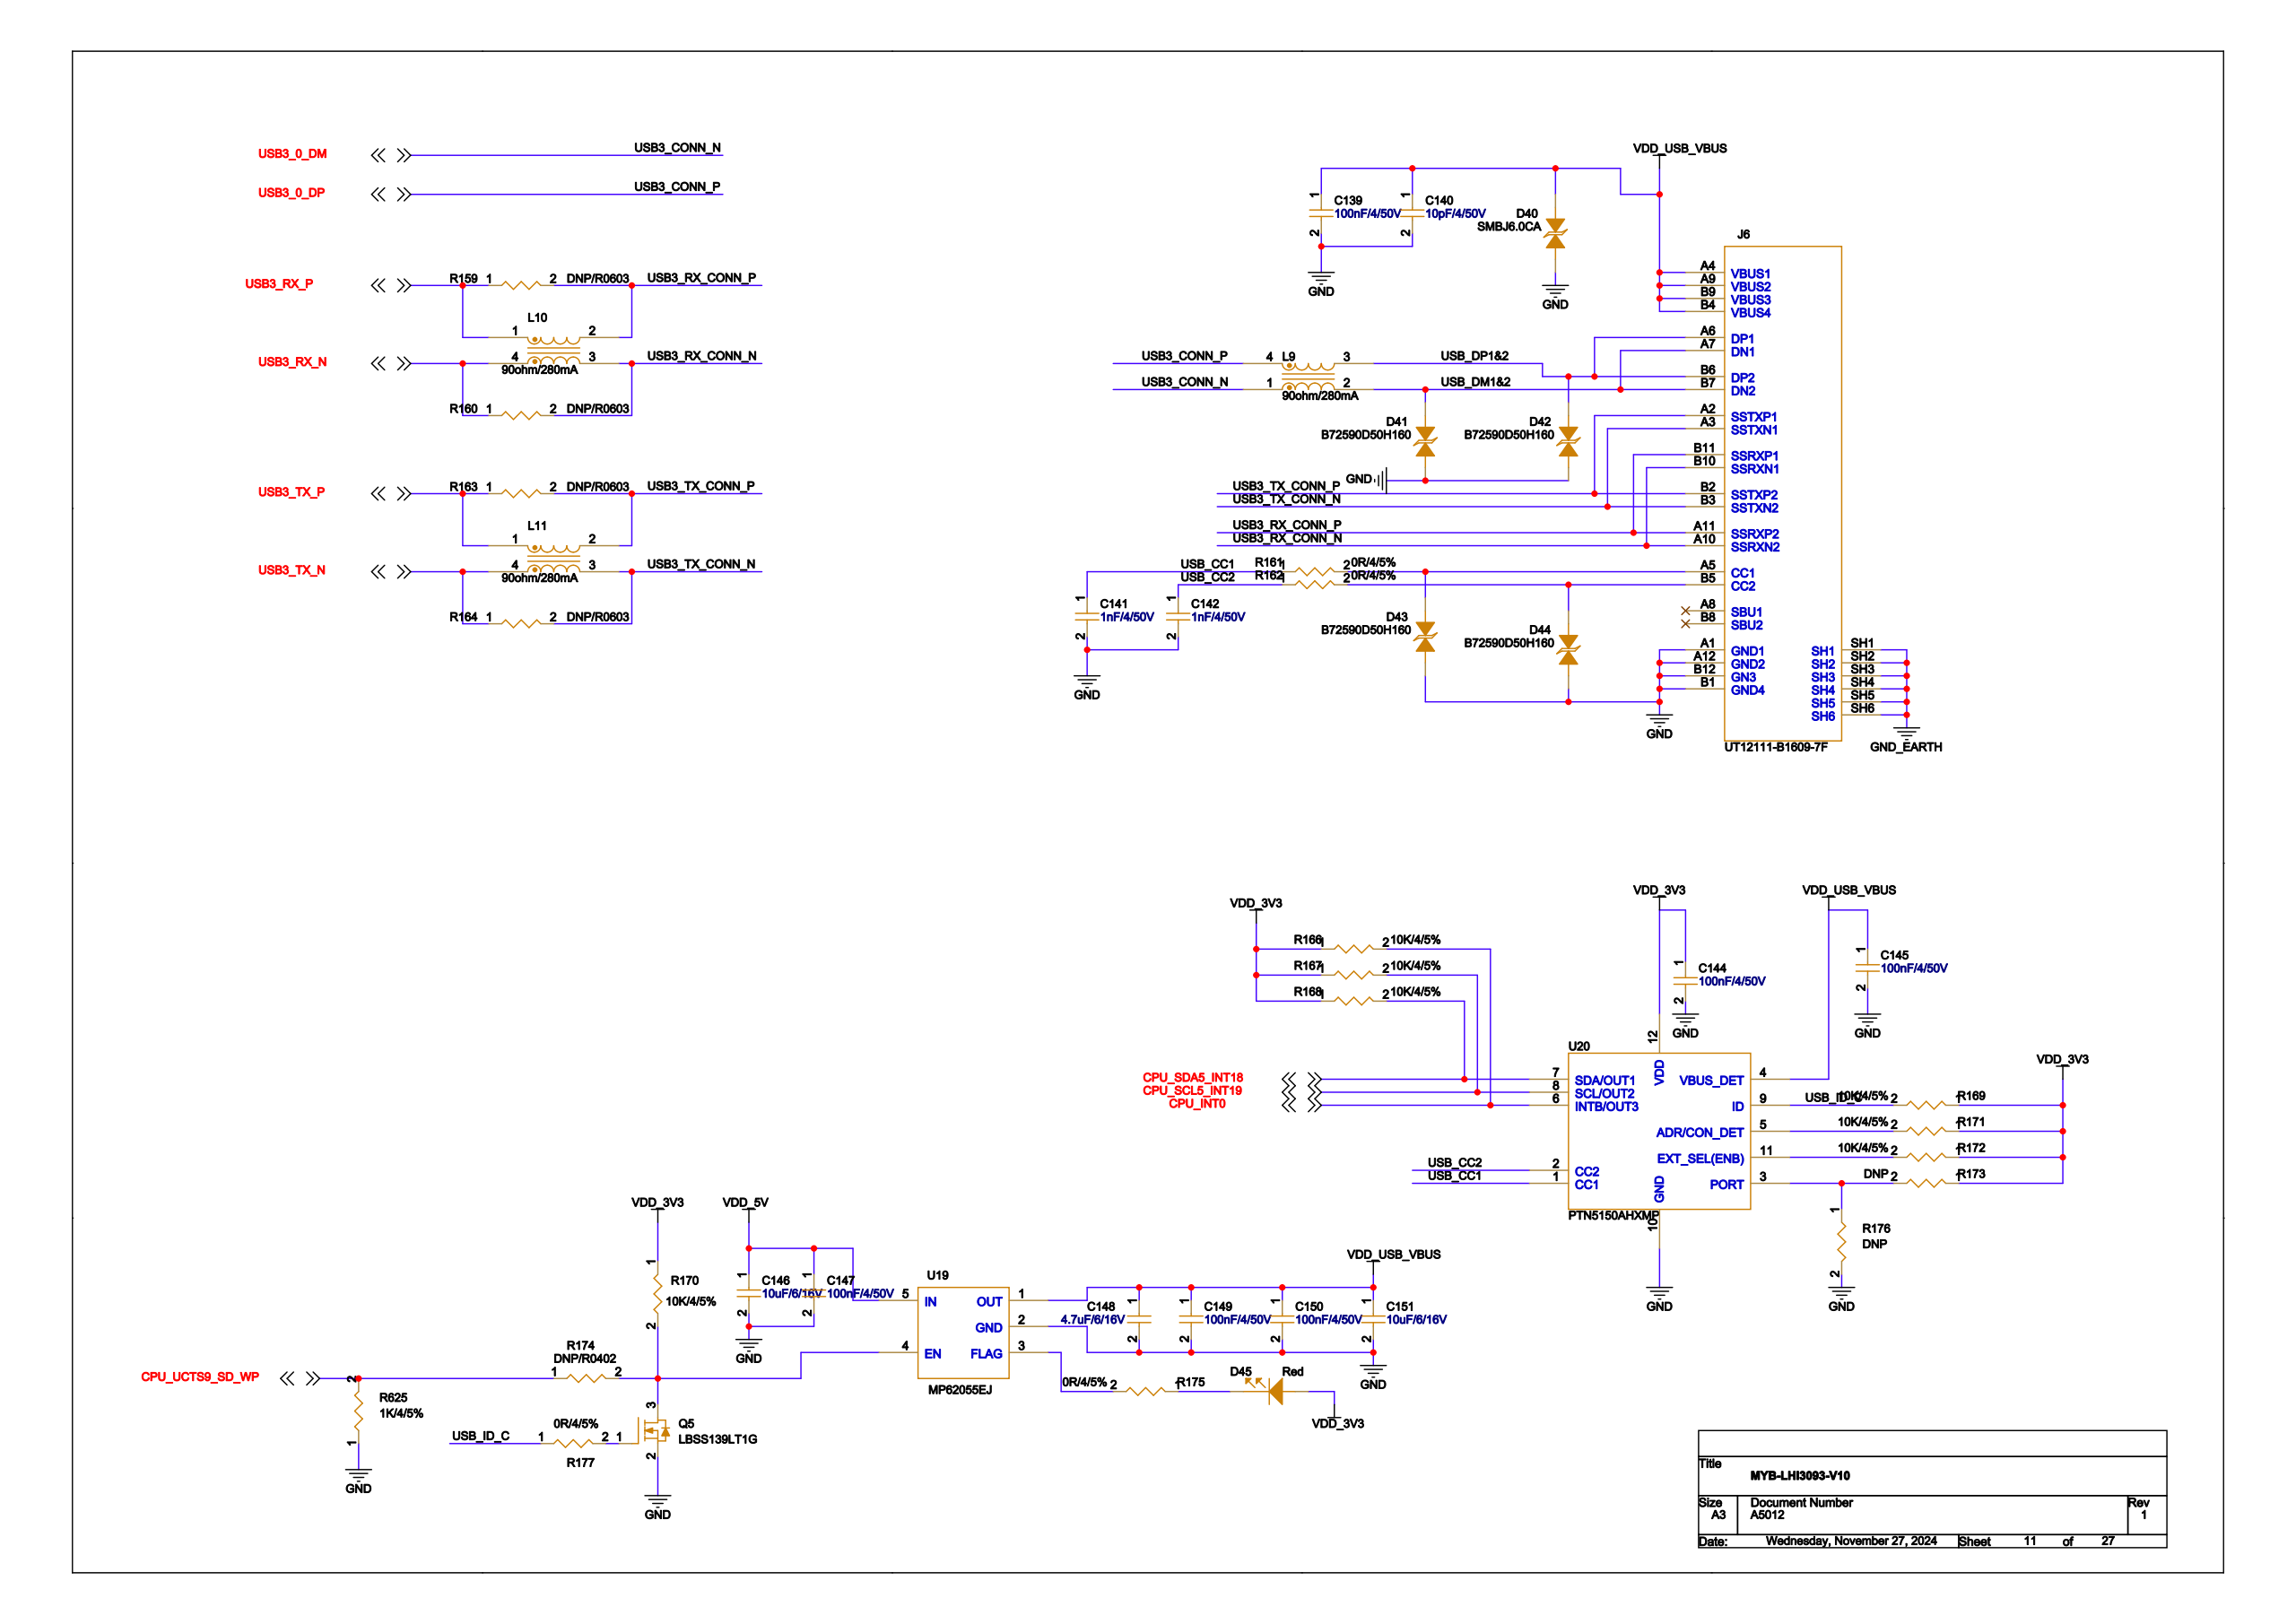Circuit board | Cadence Allegro | 1159 parts | 708 nets | one sheet of the schematic
Parts on this sheet (reference | value | footprint):
C139 | 100nF/4/50V | C0402
C140 | 10pF/4/50V | C0402
C141 | 1nF/4/50V | C0402
C142 | 1nF/4/50V | C0402
C144 | 100nF/4/50V | C0402
C145 | 100nF/4/50V | C0402
C146 | 10uF/6/16V | C0603
C147 | 100nF/4/50V | C0402
C148 | 4.7uF/6/16V | C0603
C149 | 100nF/4/50V | C0402
C150 | 100nF/4/50V | C0402
C151 | 10uF/6/16V | C0603
D40 | SMBJ6.0CA | DO-214AA
D41 | B72590D50H160 | D0402
D42 | B72590D50H160 | D0402
D43 | B72590D50H160 | D0402
D44 | B72590D50H160 | D0402
D45 | LED-SML1206 | LED0603
J6 | UT12111-B1609-7F | UT12111-B1609-7F
L9 | 90ohm/280mA | INDCM-SDCW2012
L10 | 90ohm/280mA | INDCM-SDCW2012
L11 | 90ohm/280mA | INDCM-SDCW2012
Q5 | LBSS139LT1G | SOT-23
R159 | DNP/R0603 | R0603
R160 | DNP/R0603 | R0603
R163 | DNP/R0603 | R0603
R164 | DNP/R0603 | R0603
R170 | 10K/4/5% | R0402
R174 | DNP/R0402 | R0402
R176 | DNP | R0402
R177 | 0R/4/5% | R0402
R625 | 1K/4/5% | R0402
U19 | MP62055EJ | SOT23-5
U20 | PTN5150AHXMP | X2QFN12
Nets of these parts (net: part-pin ...):
GND: C139-2 C140-2 C141-2 C142-2 C144-2 C145-2 C146-2 C147-2 C148-2 C149-2 C150-2 C151-2 D40-1 D41-1 D42-1 D43-1 D44-1 Q5-2 R176-2 R625-1 U19-2 U20-10 J6-A1 J6-A12 J6-B1 J6-B12
VDD_5V: C146-1 C147-1 U19-5
VDD_3V3: C144-1 D45-1 R170-1 U20-12
VDD_USB_VBUS: C139-1 C140-1 C145-1 C148-1 C149-1 C150-1 C151-1 D40-2 U19-1 U20-4 J6-A4 J6-A9 J6-B4 J6-B9
GND_EARTH: J6-SH1 J6-SH2 J6-SH3 J6-SH4 J6-SH5 J6-SH6
USB_CC1: C141-1 U20-1
USB_CC2: C142-1 U20-2
N14881575: D45-2
USB_DM1&2: D41-2 L9-2 J6-A7 J6-B7
USB_DP1&2: D42-2 L9-3 J6-A6 J6-B6
N14876563: D43-2 J6-A5
N14876577: D44-2 J6-B5
USB3_RX_CONN_N: L10-3 R160-2 J6-A10 J6-B10
USB3_RX_CONN_P: L10-2 R159-2 J6-A11 J6-B11
USB3_TX_CONN_N: L11-3 R164-2 J6-A3 J6-B3
USB3_TX_CONN_P: L11-2 R163-2 J6-A2 J6-B2
CPU_SCL5_INT19: U20-8
CPU_SDA5_INT18: U20-7
USB3_RX_P: L10-1 R159-1
USB3_RX_N: L10-4 R160-1
USB3_TX_P: L11-1 R163-1
USB3_TX_N: L11-4 R164-1
USB3_0_DM: L9-1
USB3_0_DP: L9-4
N14882250: Q5-3 R170-2 R174-2 U19-4
N14883738: Q5-1 R177-2
N14881563: U19-3
USB_ID_C: R177-1 U20-9
CPU_INT0: U20-6
N14879556: U20-5
N14879560: U20-11
CPU_UCTS9_SD_WP: R174-1 R625-2
N14879564: R176-1 U20-3